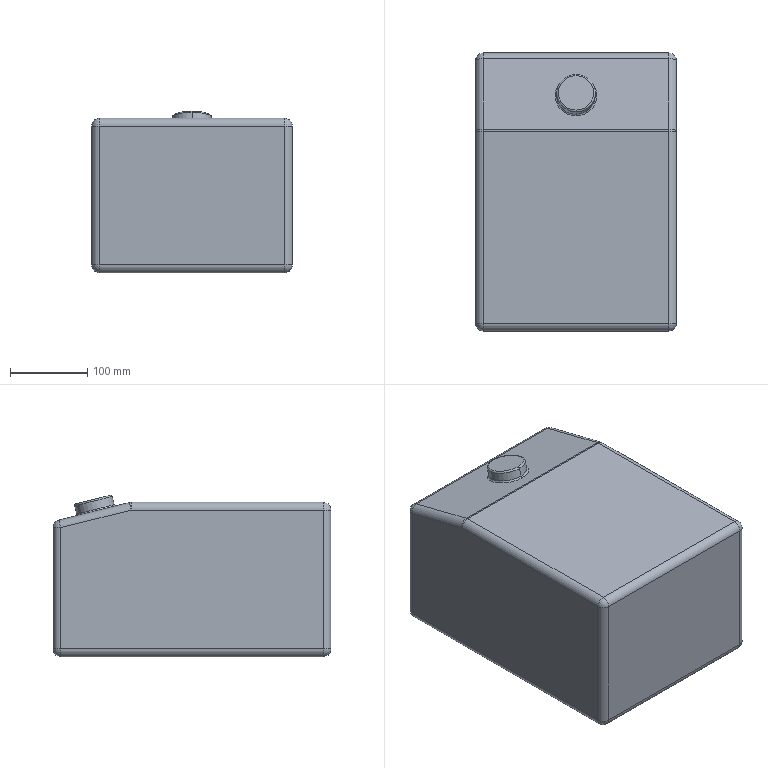Part | 1 solid | 39 faces | box 260 x 360 x 209.059 mm | volume 18358765 mm3 | cylinder 17 | sphere 10 | plane 8 | torus 4 | commonest cylinder face diameters 20 x15 50 x2
STEP:
#1=CARTESIAN_POINT('',(0.,151.932,195.417));
#2=VERTEX_POINT('',#1);
#3=CARTESIAN_POINT('',(0.,103.425,207.544));
#4=VERTEX_POINT('',#3);
#5=CARTESIAN_POINT('',(0.,127.678,201.481));
#6=DIRECTION('',(0.,-0.2425,-0.9701));
#7=DIRECTION('',(0.,-0.9701,0.2425));
#8=AXIS2_PLACEMENT_3D('',#5,#6,#7);
#9=CIRCLE('',#8,25.);
#10=EDGE_CURVE('',#2,#4,#9,.T.);
#11=ORIENTED_EDGE('',*,*,#10,.F.);
#12=CARTESIAN_POINT('',(0.,150.477,197.842));
#13=VERTEX_POINT('',#12);
#14=CARTESIAN_POINT('',(0.,149.992,195.902));
#15=DIRECTION('',(1.,0.,0.));
#16=DIRECTION('',(0.,1.,0.));
#17=AXIS2_PLACEMENT_3D('',#14,#15,#16);
#18=CIRCLE('',#17,2.);
#19=EDGE_CURVE('',#2,#13,#18,.T.);
#20=ORIENTED_EDGE('',*,*,#19,.T.);
#21=CARTESIAN_POINT('',(0.,105.85,208.999));
#22=VERTEX_POINT('',#21);
#23=CARTESIAN_POINT('',(0.,128.163,203.421));
#24=DIRECTION('',(0.,0.2425,0.9701));
#25=DIRECTION('',(0.,-0.9701,0.2425));
#26=AXIS2_PLACEMENT_3D('',#23,#24,#25);
#27=CIRCLE('',#26,23.);
#28=EDGE_CURVE('',#22,#13,#27,.T.);
#29=ORIENTED_EDGE('',*,*,#28,.F.);
#30=CARTESIAN_POINT('',(0.,105.365,207.059));
#31=DIRECTION('',(-1.,0.,0.));
#32=DIRECTION('',(0.,0.,1.));
#33=AXIS2_PLACEMENT_3D('',#30,#31,#32);
#34=CIRCLE('',#33,2.);
#35=EDGE_CURVE('',#4,#22,#34,.T.);
#36=ORIENTED_EDGE('',*,*,#35,.F.);
#37=EDGE_LOOP('',(#11,#20,#29,#36));
#38=FACE_OUTER_BOUND('',#37,.T.);
#39=CARTESIAN_POINT('',(0.,127.678,201.481));
#40=DIRECTION('',(0.,0.2425,0.9701));
#41=DIRECTION('',(0.,-0.9701,0.2425));
#42=AXIS2_PLACEMENT_3D('',#39,#40,#41);
#43=TOROIDAL_SURFACE('',#42,23.,2.);
#44=ADVANCED_FACE('',(#38),#43,.T.);
#45=CARTESIAN_POINT('',(0.,98.332,195.417));
#46=VERTEX_POINT('',#45);
#47=CARTESIAN_POINT('',(0.,150.719,182.32));
#48=VERTEX_POINT('',#47);
#49=CARTESIAN_POINT('',(0.,124.525,188.869));
#50=DIRECTION('',(0.,-0.2425,-0.9701));
#51=DIRECTION('',(0.,0.9701,-0.2425));
#52=AXIS2_PLACEMENT_3D('',#49,#50,#51);
#53=CIRCLE('',#52,27.);
#54=EDGE_CURVE('',#46,#48,#53,.T.);
#55=ORIENTED_EDGE('',*,*,#54,.F.);
#56=CARTESIAN_POINT('',(0.,100.757,196.872));
#57=VERTEX_POINT('',#56);
#58=CARTESIAN_POINT('',(0.,98.817,197.357));
#59=DIRECTION('',(1.,0.,0.));
#60=DIRECTION('',(0.,1.,0.));
#61=AXIS2_PLACEMENT_3D('',#58,#59,#60);
#62=CIRCLE('',#61,2.);
#63=EDGE_CURVE('',#46,#57,#62,.T.);
#64=ORIENTED_EDGE('',*,*,#63,.T.);
#65=CARTESIAN_POINT('',(0.,149.264,184.746));
#66=VERTEX_POINT('',#65);
#67=CARTESIAN_POINT('',(0.,125.01,190.809));
#68=DIRECTION('',(0.,0.2425,0.9701));
#69=DIRECTION('',(0.,0.9701,-0.2425));
#70=AXIS2_PLACEMENT_3D('',#67,#68,#69);
#71=CIRCLE('',#70,25.);
#72=EDGE_CURVE('',#66,#57,#71,.T.);
#73=ORIENTED_EDGE('',*,*,#72,.F.);
#74=CARTESIAN_POINT('',(0.,151.204,184.26));
#75=DIRECTION('',(-1.,0.,0.));
#76=DIRECTION('',(0.,0.,1.));
#77=AXIS2_PLACEMENT_3D('',#74,#75,#76);
#78=CIRCLE('',#77,2.);
#79=EDGE_CURVE('',#48,#66,#78,.T.);
#80=ORIENTED_EDGE('',*,*,#79,.F.);
#81=EDGE_LOOP('',(#55,#64,#73,#80));
#82=FACE_OUTER_BOUND('',#81,.T.);
#83=CARTESIAN_POINT('',(0.,125.01,190.809));
#84=DIRECTION('',(0.,-0.2425,-0.9701));
#85=DIRECTION('',(0.,0.9701,-0.2425));
#86=AXIS2_PLACEMENT_3D('',#83,#84,#85);
#87=TOROIDAL_SURFACE('',#86,27.,2.);
#88=ADVANCED_FACE('',(#82),#87,.F.);
#89=ORIENTED_EDGE('',*,*,#10,.T.);
#90=CARTESIAN_POINT('',(0.,103.91,209.484));
#91=DIRECTION('',(0.,-0.2425,-0.9701));
#92=VECTOR('',#91,1000.);
#93=LINE('',#90,#92);
#94=EDGE_CURVE('',#4,#57,#93,.T.);
#95=ORIENTED_EDGE('',*,*,#94,.T.);
#96=CARTESIAN_POINT('',(0.,125.01,190.809));
#97=DIRECTION('',(0.,0.2425,0.9701));
#98=DIRECTION('',(0.,0.9701,-0.2425));
#99=AXIS2_PLACEMENT_3D('',#96,#97,#98);
#100=CIRCLE('',#99,25.);
#101=EDGE_CURVE('',#57,#66,#100,.T.);
#102=ORIENTED_EDGE('',*,*,#101,.T.);
#103=CARTESIAN_POINT('',(0.,152.417,197.357));
#104=DIRECTION('',(0.,-0.2425,-0.9701));
#105=VECTOR('',#104,1000.);
#106=LINE('',#103,#105);
#107=EDGE_CURVE('',#2,#66,#106,.T.);
#108=ORIENTED_EDGE('',*,*,#107,.F.);
#109=EDGE_LOOP('',(#89,#95,#102,#108));
#110=FACE_OUTER_BOUND('',#109,.T.);
#111=CARTESIAN_POINT('',(0.,128.163,203.421));
#112=DIRECTION('',(0.,-0.2425,-0.9701));
#113=DIRECTION('',(0.,0.9701,-0.2425));
#114=AXIS2_PLACEMENT_3D('',#111,#112,#113);
#115=CYLINDRICAL_SURFACE('',#114,25.);
#116=ADVANCED_FACE('',(#110),#115,.T.);
#117=CARTESIAN_POINT('',(130.,-170.,10.));
#118=VERTEX_POINT('',#117);
#119=CARTESIAN_POINT('',(130.,170.,10.));
#120=VERTEX_POINT('',#119);
#121=CARTESIAN_POINT('',(130.,180.,10.));
#122=DIRECTION('',(0.,1.,0.));
#123=VECTOR('',#122,1000.);
#124=LINE('',#121,#123);
#125=EDGE_CURVE('',#118,#120,#124,.T.);
#126=ORIENTED_EDGE('',*,*,#125,.T.);
#127=CARTESIAN_POINT('',(130.,170.,167.192));
#128=VERTEX_POINT('',#127);
#129=CARTESIAN_POINT('',(130.,170.,200.));
#130=DIRECTION('',(0.,0.,1.));
#131=VECTOR('',#130,1000.);
#132=LINE('',#129,#131);
#133=EDGE_CURVE('',#120,#128,#132,.T.);
#134=ORIENTED_EDGE('',*,*,#133,.T.);
#135=CARTESIAN_POINT('',(130.,78.769,190.));
#136=VERTEX_POINT('',#135);
#137=CARTESIAN_POINT('',(130.,-167.131,251.475));
#138=DIRECTION('',(0.,-0.9701,0.2425));
#139=VECTOR('',#138,1000.);
#140=LINE('',#137,#139);
#141=EDGE_CURVE('',#128,#136,#140,.T.);
#142=ORIENTED_EDGE('',*,*,#141,.T.);
#143=CARTESIAN_POINT('',(130.,-170.,190.));
#144=VERTEX_POINT('',#143);
#145=CARTESIAN_POINT('',(130.,-180.,190.));
#146=DIRECTION('',(0.,-1.,0.));
#147=VECTOR('',#146,1000.);
#148=LINE('',#145,#147);
#149=EDGE_CURVE('',#136,#144,#148,.T.);
#150=ORIENTED_EDGE('',*,*,#149,.T.);
#151=CARTESIAN_POINT('',(130.,-170.,200.));
#152=DIRECTION('',(0.,0.,-1.));
#153=VECTOR('',#152,1000.);
#154=LINE('',#151,#153);
#155=EDGE_CURVE('',#144,#118,#154,.T.);
#156=ORIENTED_EDGE('',*,*,#155,.T.);
#157=EDGE_LOOP('',(#126,#134,#142,#150,#156));
#158=FACE_OUTER_BOUND('',#157,.T.);
#159=CARTESIAN_POINT('',(130.,-180.,200.));
#160=DIRECTION('',(-1.,0.,0.));
#161=DIRECTION('',(0.,0.,1.));
#162=AXIS2_PLACEMENT_3D('',#159,#160,#161);
#163=PLANE('',#162);
#164=ADVANCED_FACE('',(#158),#163,.F.);
#165=CARTESIAN_POINT('',(-120.,180.,167.192));
#166=VERTEX_POINT('',#165);
#167=CARTESIAN_POINT('',(120.,180.,167.192));
#168=VERTEX_POINT('',#167);
#169=CARTESIAN_POINT('',(-130.,180.,167.192));
#170=DIRECTION('',(1.,0.,0.));
#171=VECTOR('',#170,1000.);
#172=LINE('',#169,#171);
#173=EDGE_CURVE('',#166,#168,#172,.T.);
#174=ORIENTED_EDGE('',*,*,#173,.T.);
#175=CARTESIAN_POINT('',(120.,180.,10.));
#176=VERTEX_POINT('',#175);
#177=CARTESIAN_POINT('',(120.,180.,200.));
#178=DIRECTION('',(0.,0.,-1.));
#179=VECTOR('',#178,1000.);
#180=LINE('',#177,#179);
#181=EDGE_CURVE('',#168,#176,#180,.T.);
#182=ORIENTED_EDGE('',*,*,#181,.T.);
#183=CARTESIAN_POINT('',(-120.,180.,10.));
#184=VERTEX_POINT('',#183);
#185=CARTESIAN_POINT('',(-130.,180.,10.));
#186=DIRECTION('',(-1.,0.,0.));
#187=VECTOR('',#186,1000.);
#188=LINE('',#185,#187);
#189=EDGE_CURVE('',#176,#184,#188,.T.);
#190=ORIENTED_EDGE('',*,*,#189,.T.);
#191=CARTESIAN_POINT('',(-120.,180.,200.));
#192=DIRECTION('',(0.,0.,1.));
#193=VECTOR('',#192,1000.);
#194=LINE('',#191,#193);
#195=EDGE_CURVE('',#184,#166,#194,.T.);
#196=ORIENTED_EDGE('',*,*,#195,.T.);
#197=EDGE_LOOP('',(#174,#182,#190,#196));
#198=FACE_OUTER_BOUND('',#197,.T.);
#199=CARTESIAN_POINT('',(-130.,180.,200.));
#200=DIRECTION('',(0.,-1.,0.));
#201=DIRECTION('',(0.,0.,-1.));
#202=AXIS2_PLACEMENT_3D('',#199,#200,#201);
#203=PLANE('',#202);
#204=ADVANCED_FACE('',(#198),#203,.F.);
#205=CARTESIAN_POINT('',(-130.,170.,10.));
#206=VERTEX_POINT('',#205);
#207=CARTESIAN_POINT('',(-130.,-170.,10.));
#208=VERTEX_POINT('',#207);
#209=CARTESIAN_POINT('',(-130.,-180.,10.));
#210=DIRECTION('',(0.,-1.,0.));
#211=VECTOR('',#210,1000.);
#212=LINE('',#209,#211);
#213=EDGE_CURVE('',#206,#208,#212,.T.);
#214=ORIENTED_EDGE('',*,*,#213,.T.);
#215=CARTESIAN_POINT('',(-130.,-170.,190.));
#216=VERTEX_POINT('',#215);
#217=CARTESIAN_POINT('',(-130.,-170.,200.));
#218=DIRECTION('',(0.,0.,1.));
#219=VECTOR('',#218,1000.);
#220=LINE('',#217,#219);
#221=EDGE_CURVE('',#208,#216,#220,.T.);
#222=ORIENTED_EDGE('',*,*,#221,.T.);
#223=CARTESIAN_POINT('',(-130.,78.769,190.));
#224=VERTEX_POINT('',#223);
#225=CARTESIAN_POINT('',(-130.,-180.,190.));
#226=DIRECTION('',(0.,1.,0.));
#227=VECTOR('',#226,1000.);
#228=LINE('',#225,#227);
#229=EDGE_CURVE('',#216,#224,#228,.T.);
#230=ORIENTED_EDGE('',*,*,#229,.T.);
#231=CARTESIAN_POINT('',(-130.,170.,167.192));
#232=VERTEX_POINT('',#231);
#233=CARTESIAN_POINT('',(-130.,-167.131,251.475));
#234=DIRECTION('',(0.,0.9701,-0.2425));
#235=VECTOR('',#234,1000.);
#236=LINE('',#233,#235);
#237=EDGE_CURVE('',#224,#232,#236,.T.);
#238=ORIENTED_EDGE('',*,*,#237,.T.);
#239=CARTESIAN_POINT('',(-130.,170.,200.));
#240=DIRECTION('',(0.,0.,-1.));
#241=VECTOR('',#240,1000.);
#242=LINE('',#239,#241);
#243=EDGE_CURVE('',#232,#206,#242,.T.);
#244=ORIENTED_EDGE('',*,*,#243,.T.);
#245=EDGE_LOOP('',(#214,#222,#230,#238,#244));
#246=FACE_OUTER_BOUND('',#245,.T.);
#247=CARTESIAN_POINT('',(-130.,-180.,200.));
#248=DIRECTION('',(1.,0.,0.));
#249=DIRECTION('',(0.,0.,-1.));
#250=AXIS2_PLACEMENT_3D('',#247,#248,#249);
#251=PLANE('',#250);
#252=ADVANCED_FACE('',(#246),#251,.F.);
#253=CARTESIAN_POINT('',(120.,-180.,190.));
#254=VERTEX_POINT('',#253);
#255=CARTESIAN_POINT('',(-120.,-180.,190.));
#256=VERTEX_POINT('',#255);
#257=CARTESIAN_POINT('',(-130.,-180.,190.));
#258=DIRECTION('',(-1.,0.,0.));
#259=VECTOR('',#258,1000.);
#260=LINE('',#257,#259);
#261=EDGE_CURVE('',#254,#256,#260,.T.);
#262=ORIENTED_EDGE('',*,*,#261,.T.);
#263=CARTESIAN_POINT('',(-120.,-180.,10.));
#264=VERTEX_POINT('',#263);
#265=CARTESIAN_POINT('',(-120.,-180.,200.));
#266=DIRECTION('',(0.,0.,-1.));
#267=VECTOR('',#266,1000.);
#268=LINE('',#265,#267);
#269=EDGE_CURVE('',#256,#264,#268,.T.);
#270=ORIENTED_EDGE('',*,*,#269,.T.);
#271=CARTESIAN_POINT('',(120.,-180.,10.));
#272=VERTEX_POINT('',#271);
#273=CARTESIAN_POINT('',(130.,-180.,10.));
#274=DIRECTION('',(1.,0.,0.));
#275=VECTOR('',#274,1000.);
#276=LINE('',#273,#275);
#277=EDGE_CURVE('',#264,#272,#276,.T.);
#278=ORIENTED_EDGE('',*,*,#277,.T.);
#279=CARTESIAN_POINT('',(120.,-180.,200.));
#280=DIRECTION('',(0.,0.,1.));
#281=VECTOR('',#280,1000.);
#282=LINE('',#279,#281);
#283=EDGE_CURVE('',#272,#254,#282,.T.);
#284=ORIENTED_EDGE('',*,*,#283,.T.);
#285=EDGE_LOOP('',(#262,#270,#278,#284));
#286=FACE_OUTER_BOUND('',#285,.T.);
#287=CARTESIAN_POINT('',(-130.,-180.,200.));
#288=DIRECTION('',(0.,1.,0.));
#289=DIRECTION('',(0.,0.,1.));
#290=AXIS2_PLACEMENT_3D('',#287,#288,#289);
#291=PLANE('',#290);
#292=ADVANCED_FACE('',(#286),#291,.F.);
#293=CARTESIAN_POINT('',(-120.,78.769,200.));
#294=VERTEX_POINT('',#293);
#295=CARTESIAN_POINT('',(-120.,-170.,200.));
#296=VERTEX_POINT('',#295);
#297=CARTESIAN_POINT('',(-120.,0.,200.));
#298=DIRECTION('',(0.,-1.,0.));
#299=VECTOR('',#298,1000.);
#300=LINE('',#297,#299);
#301=EDGE_CURVE('',#294,#296,#300,.T.);
#302=ORIENTED_EDGE('',*,*,#301,.T.);
#303=CARTESIAN_POINT('',(120.,-170.,200.));
#304=VERTEX_POINT('',#303);
#305=CARTESIAN_POINT('',(0.,-170.,200.));
#306=DIRECTION('',(1.,0.,0.));
#307=VECTOR('',#306,1000.);
#308=LINE('',#305,#307);
#309=EDGE_CURVE('',#296,#304,#308,.T.);
#310=ORIENTED_EDGE('',*,*,#309,.T.);
#311=CARTESIAN_POINT('',(120.,78.769,200.));
#312=VERTEX_POINT('',#311);
#313=CARTESIAN_POINT('',(120.,0.,200.));
#314=DIRECTION('',(0.,1.,0.));
#315=VECTOR('',#314,1000.);
#316=LINE('',#313,#315);
#317=EDGE_CURVE('',#304,#312,#316,.T.);
#318=ORIENTED_EDGE('',*,*,#317,.T.);
#319=CARTESIAN_POINT('',(0.,78.769,200.));
#320=DIRECTION('',(-1.,0.,0.));
#321=VECTOR('',#320,1000.);
#322=LINE('',#319,#321);
#323=EDGE_CURVE('',#312,#294,#322,.T.);
#324=ORIENTED_EDGE('',*,*,#323,.T.);
#325=EDGE_LOOP('',(#302,#310,#318,#324));
#326=FACE_OUTER_BOUND('',#325,.T.);
#327=CARTESIAN_POINT('',(0.,0.,200.));
#328=DIRECTION('',(0.,0.,-1.));
#329=DIRECTION('',(-1.,0.,0.));
#330=AXIS2_PLACEMENT_3D('',#327,#328,#329);
#331=PLANE('',#330);
#332=ADVANCED_FACE('',(#326),#331,.F.);
#333=CARTESIAN_POINT('',(-120.,-170.,0.));
#334=VERTEX_POINT('',#333);
#335=CARTESIAN_POINT('',(-120.,170.,0.));
#336=VERTEX_POINT('',#335);
#337=CARTESIAN_POINT('',(-120.,180.,0.));
#338=DIRECTION('',(0.,1.,0.));
#339=VECTOR('',#338,1000.);
#340=LINE('',#337,#339);
#341=EDGE_CURVE('',#334,#336,#340,.T.);
#342=ORIENTED_EDGE('',*,*,#341,.T.);
#343=CARTESIAN_POINT('',(120.,170.,0.));
#344=VERTEX_POINT('',#343);
#345=CARTESIAN_POINT('',(130.,170.,0.));
#346=DIRECTION('',(1.,0.,0.));
#347=VECTOR('',#346,1000.);
#348=LINE('',#345,#347);
#349=EDGE_CURVE('',#336,#344,#348,.T.);
#350=ORIENTED_EDGE('',*,*,#349,.T.);
#351=CARTESIAN_POINT('',(120.,-170.,0.));
#352=VERTEX_POINT('',#351);
#353=CARTESIAN_POINT('',(120.,-180.,0.));
#354=DIRECTION('',(0.,-1.,0.));
#355=VECTOR('',#354,1000.);
#356=LINE('',#353,#355);
#357=EDGE_CURVE('',#344,#352,#356,.T.);
#358=ORIENTED_EDGE('',*,*,#357,.T.);
#359=CARTESIAN_POINT('',(-130.,-170.,0.));
#360=DIRECTION('',(-1.,0.,0.));
#361=VECTOR('',#360,1000.);
#362=LINE('',#359,#361);
#363=EDGE_CURVE('',#352,#334,#362,.T.);
#364=ORIENTED_EDGE('',*,*,#363,.T.);
#365=EDGE_LOOP('',(#342,#350,#358,#364));
#366=FACE_OUTER_BOUND('',#365,.T.);
#367=CARTESIAN_POINT('',(0.,0.,0.));
#368=DIRECTION('',(0.,0.,-1.));
#369=DIRECTION('',(-1.,0.,0.));
#370=AXIS2_PLACEMENT_3D('',#367,#368,#369);
#371=PLANE('',#370);
#372=ADVANCED_FACE('',(#366),#371,.T.);
#373=CARTESIAN_POINT('',(-120.,81.194,199.701));
#374=VERTEX_POINT('',#373);
#375=CARTESIAN_POINT('',(120.,81.194,199.701));
#376=VERTEX_POINT('',#375);
#377=CARTESIAN_POINT('',(130.,81.194,199.701));
#378=DIRECTION('',(1.,0.,0.));
#379=VECTOR('',#378,1000.);
#380=LINE('',#377,#379);
#381=EDGE_CURVE('',#374,#376,#380,.T.);
#382=ORIENTED_EDGE('',*,*,#381,.T.);
#383=CARTESIAN_POINT('',(120.,172.425,176.894));
#384=VERTEX_POINT('',#383);
#385=CARTESIAN_POINT('',(120.,180.,175.));
#386=DIRECTION('',(0.,0.9701,-0.2425));
#387=VECTOR('',#386,1000.);
#388=LINE('',#385,#387);
#389=EDGE_CURVE('',#376,#384,#388,.T.);
#390=ORIENTED_EDGE('',*,*,#389,.T.);
#391=CARTESIAN_POINT('',(-120.,172.425,176.894));
#392=VERTEX_POINT('',#391);
#393=CARTESIAN_POINT('',(130.,172.425,176.894));
#394=DIRECTION('',(-1.,0.,0.));
#395=VECTOR('',#394,1000.);
#396=LINE('',#393,#395);
#397=EDGE_CURVE('',#384,#392,#396,.T.);
#398=ORIENTED_EDGE('',*,*,#397,.T.);
#399=CARTESIAN_POINT('',(-120.,180.,175.));
#400=DIRECTION('',(0.,-0.9701,0.2425));
#401=VECTOR('',#400,1000.);
#402=LINE('',#399,#401);
#403=EDGE_CURVE('',#392,#374,#402,.T.);
#404=ORIENTED_EDGE('',*,*,#403,.T.);
#405=EDGE_LOOP('',(#382,#390,#398,#404));
#406=FACE_OUTER_BOUND('',#405,.T.);
#407=CARTESIAN_POINT('',(0.,124.525,188.869));
#408=DIRECTION('',(0.,-0.2425,-0.9701));
#409=DIRECTION('',(0.,0.9701,-0.2425));
#410=AXIS2_PLACEMENT_3D('',#407,#408,#409);
#411=CIRCLE('',#410,27.);
#412=EDGE_CURVE('',#48,#46,#411,.T.);
#413=ORIENTED_EDGE('',*,*,#412,.T.);
#414=ORIENTED_EDGE('',*,*,#54,.T.);
#415=EDGE_LOOP('',(#413,#414));
#416=FACE_BOUND('',#415,.T.);
#417=CARTESIAN_POINT('',(130.,180.,175.));
#418=DIRECTION('',(0.,-0.2425,-0.9701));
#419=DIRECTION('',(0.,0.9701,-0.2425));
#420=AXIS2_PLACEMENT_3D('',#417,#418,#419);
#421=PLANE('',#420);
#422=ADVANCED_FACE('',(#406,#416),#421,.F.);
#423=ORIENTED_EDGE('',*,*,#277,.F.);
#424=CARTESIAN_POINT('',(-120.,-170.,10.));
#425=DIRECTION('',(1.,0.,0.));
#426=DIRECTION('',(0.,0.,1.));
#427=AXIS2_PLACEMENT_3D('',#424,#425,#426);
#428=CIRCLE('',#427,10.);
#429=EDGE_CURVE('',#264,#334,#428,.T.);
#430=ORIENTED_EDGE('',*,*,#429,.T.);
#431=ORIENTED_EDGE('',*,*,#363,.F.);
#432=CARTESIAN_POINT('',(120.,-170.,10.));
#433=DIRECTION('',(-1.,0.,0.));
#434=DIRECTION('',(0.,0.,1.));
#435=AXIS2_PLACEMENT_3D('',#432,#433,#434);
#436=CIRCLE('',#435,10.);
#437=EDGE_CURVE('',#352,#272,#436,.T.);
#438=ORIENTED_EDGE('',*,*,#437,.T.);
#439=EDGE_LOOP('',(#423,#430,#431,#438));
#440=FACE_OUTER_BOUND('',#439,.T.);
#441=CARTESIAN_POINT('',(-130.,-170.,10.));
#442=DIRECTION('',(-1.,0.,0.));
#443=DIRECTION('',(0.,0.,1.));
#444=AXIS2_PLACEMENT_3D('',#441,#442,#443);
#445=CYLINDRICAL_SURFACE('',#444,10.);
#446=ADVANCED_FACE('',(#440),#445,.T.);
#447=ORIENTED_EDGE('',*,*,#125,.F.);
#448=CARTESIAN_POINT('',(120.,-170.,10.));
#449=DIRECTION('',(0.,1.,0.));
#450=DIRECTION('',(0.,0.,-1.));
#451=AXIS2_PLACEMENT_3D('',#448,#449,#450);
#452=CIRCLE('',#451,10.);
#453=EDGE_CURVE('',#118,#352,#452,.T.);
#454=ORIENTED_EDGE('',*,*,#453,.T.);
#455=ORIENTED_EDGE('',*,*,#357,.F.);
#456=CARTESIAN_POINT('',(120.,170.,10.));
#457=DIRECTION('',(0.,-1.,0.));
#458=DIRECTION('',(0.,0.,-1.));
#459=AXIS2_PLACEMENT_3D('',#456,#457,#458);
#460=CIRCLE('',#459,10.);
#461=EDGE_CURVE('',#344,#120,#460,.T.);
#462=ORIENTED_EDGE('',*,*,#461,.T.);
#463=EDGE_LOOP('',(#447,#454,#455,#462));
#464=FACE_OUTER_BOUND('',#463,.T.);
#465=CARTESIAN_POINT('',(120.,-180.,10.));
#466=DIRECTION('',(0.,-1.,0.));
#467=DIRECTION('',(0.,0.,-1.));
#468=AXIS2_PLACEMENT_3D('',#465,#466,#467);
#469=CYLINDRICAL_SURFACE('',#468,10.);
#470=ADVANCED_FACE('',(#464),#469,.T.);
#471=ORIENTED_EDGE('',*,*,#341,.F.);
#472=CARTESIAN_POINT('',(-120.,-170.,10.));
#473=DIRECTION('',(0.,1.,0.));
#474=DIRECTION('',(0.,0.,1.));
#475=AXIS2_PLACEMENT_3D('',#472,#473,#474);
#476=CIRCLE('',#475,10.);
#477=EDGE_CURVE('',#334,#208,#476,.T.);
#478=ORIENTED_EDGE('',*,*,#477,.T.);
#479=ORIENTED_EDGE('',*,*,#213,.F.);
#480=CARTESIAN_POINT('',(-120.,170.,10.));
#481=DIRECTION('',(0.,-1.,0.));
#482=DIRECTION('',(0.,0.,1.));
#483=AXIS2_PLACEMENT_3D('',#480,#481,#482);
#484=CIRCLE('',#483,10.);
#485=EDGE_CURVE('',#206,#336,#484,.T.);
#486=ORIENTED_EDGE('',*,*,#485,.T.);
#487=EDGE_LOOP('',(#471,#478,#479,#486));
#488=FACE_OUTER_BOUND('',#487,.T.);
#489=CARTESIAN_POINT('',(-120.,-180.,10.));
#490=DIRECTION('',(0.,1.,0.));
#491=DIRECTION('',(0.,0.,1.));
#492=AXIS2_PLACEMENT_3D('',#489,#490,#491);
#493=CYLINDRICAL_SURFACE('',#492,10.);
#494=ADVANCED_FACE('',(#488),#493,.T.);
#495=ORIENTED_EDGE('',*,*,#189,.F.);
#496=CARTESIAN_POINT('',(120.,170.,10.));
#497=DIRECTION('',(-1.,0.,0.));
#498=DIRECTION('',(0.,0.,-1.));
#499=AXIS2_PLACEMENT_3D('',#496,#497,#498);
#500=CIRCLE('',#499,10.);
#501=EDGE_CURVE('',#176,#344,#500,.T.);
#502=ORIENTED_EDGE('',*,*,#501,.T.);
#503=ORIENTED_EDGE('',*,*,#349,.F.);
#504=CARTESIAN_POINT('',(-120.,170.,10.));
#505=DIRECTION('',(1.,0.,0.));
#506=DIRECTION('',(0.,0.,-1.));
#507=AXIS2_PLACEMENT_3D('',#504,#505,#506);
#508=CIRCLE('',#507,10.);
#509=EDGE_CURVE('',#336,#184,#508,.T.);
#510=ORIENTED_EDGE('',*,*,#509,.T.);
#511=EDGE_LOOP('',(#495,#502,#503,#510));
#512=FACE_OUTER_BOUND('',#511,.T.);
#513=CARTESIAN_POINT('',(-130.,170.,10.));
#514=DIRECTION('',(1.,0.,0.));
#515=DIRECTION('',(0.,0.,-1.));
#516=AXIS2_PLACEMENT_3D('',#513,#514,#515);
#517=CYLINDRICAL_SURFACE('',#516,10.);
#518=ADVANCED_FACE('',(#512),#517,.T.);
#519=ORIENTED_EDGE('',*,*,#94,.F.);
#520=CARTESIAN_POINT('',(0.,127.678,201.481));
#521=DIRECTION('',(0.,-0.2425,-0.9701));
#522=DIRECTION('',(0.,-0.9701,0.2425));
#523=AXIS2_PLACEMENT_3D('',#520,#521,#522);
#524=CIRCLE('',#523,25.);
#525=EDGE_CURVE('',#4,#2,#524,.T.);
#526=ORIENTED_EDGE('',*,*,#525,.T.);
#527=ORIENTED_EDGE('',*,*,#107,.T.);
#528=ORIENTED_EDGE('',*,*,#72,.T.);
#529=EDGE_LOOP('',(#519,#526,#527,#528));
#530=FACE_OUTER_BOUND('',#529,.T.);
#531=CARTESIAN_POINT('',(0.,128.163,203.421));
#532=DIRECTION('',(0.,-0.2425,-0.9701));
#533=DIRECTION('',(0.,0.9701,-0.2425));
#534=AXIS2_PLACEMENT_3D('',#531,#532,#533);
#535=CYLINDRICAL_SURFACE('',#534,25.);
#536=ADVANCED_FACE('',(#530),#535,.T.);
#537=ORIENTED_EDGE('',*,*,#28,.T.);
#538=CARTESIAN_POINT('',(0.,128.163,203.421));
#539=DIRECTION('',(0.,0.2425,0.9701));
#540=DIRECTION('',(0.,-0.9701,0.2425));
#541=AXIS2_PLACEMENT_3D('',#538,#539,#540);
#542=CIRCLE('',#541,23.);
#543=EDGE_CURVE('',#13,#22,#542,.T.);
#544=ORIENTED_EDGE('',*,*,#543,.T.);
#545=EDGE_LOOP('',(#537,#544));
#546=FACE_OUTER_BOUND('',#545,.T.);
#547=CARTESIAN_POINT('',(0.,128.163,203.421));
#548=DIRECTION('',(0.,0.2425,0.9701));
#549=DIRECTION('',(0.,-0.9701,0.2425));
#550=AXIS2_PLACEMENT_3D('',#547,#548,#549);
#551=PLANE('',#550);
#552=ADVANCED_FACE('',(#546),#551,.T.);
#553=ORIENTED_EDGE('',*,*,#63,.F.);
#554=ORIENTED_EDGE('',*,*,#412,.F.);
#555=ORIENTED_EDGE('',*,*,#79,.T.);
#556=ORIENTED_EDGE('',*,*,#101,.F.);
#557=EDGE_LOOP('',(#553,#554,#555,#556));
#558=FACE_OUTER_BOUND('',#557,.T.);
#559=CARTESIAN_POINT('',(0.,125.01,190.809));
#560=DIRECTION('',(0.,-0.2425,-0.9701));
#561=DIRECTION('',(0.,0.9701,-0.2425));
#562=AXIS2_PLACEMENT_3D('',#559,#560,#561);
#563=TOROIDAL_SURFACE('',#562,27.,2.);
#564=ADVANCED_FACE('',(#558),#563,.F.);
#565=ORIENTED_EDGE('',*,*,#19,.F.);
#566=ORIENTED_EDGE('',*,*,#525,.F.);
#567=ORIENTED_EDGE('',*,*,#35,.T.);
#568=ORIENTED_EDGE('',*,*,#543,.F.);
#569=EDGE_LOOP('',(#565,#566,#567,#568));
#570=FACE_OUTER_BOUND('',#569,.T.);
#571=CARTESIAN_POINT('',(0.,127.678,201.481));
#572=DIRECTION('',(0.,0.2425,0.9701));
#573=DIRECTION('',(0.,-0.9701,0.2425));
#574=AXIS2_PLACEMENT_3D('',#571,#572,#573);
#575=TOROIDAL_SURFACE('',#574,23.,2.);
#576=ADVANCED_FACE('',(#570),#575,.T.);
#577=ORIENTED_EDGE('',*,*,#461,.F.);
#578=ORIENTED_EDGE('',*,*,#501,.F.);
#579=CARTESIAN_POINT('',(120.,170.,10.));
#580=DIRECTION('',(0.,0.,1.));
#581=DIRECTION('',(1.,0.,0.));
#582=AXIS2_PLACEMENT_3D('',#579,#580,#581);
#583=CIRCLE('',#582,10.);
#584=EDGE_CURVE('',#120,#176,#583,.T.);
#585=ORIENTED_EDGE('',*,*,#584,.F.);
#586=EDGE_LOOP('',(#577,#578,#585));
#587=FACE_OUTER_BOUND('',#586,.T.);
#588=CARTESIAN_POINT('',(120.,170.,10.));
#589=DIRECTION('',(0.,1.,0.));
#590=DIRECTION('',(1.,0.,0.));
#591=AXIS2_PLACEMENT_3D('',#588,#589,#590);
#592=SPHERICAL_SURFACE('',#591,10.);
#593=ADVANCED_FACE('',(#587),#592,.T.);
#594=ORIENTED_EDGE('',*,*,#584,.T.);
#595=ORIENTED_EDGE('',*,*,#181,.F.);
#596=CARTESIAN_POINT('',(120.,170.,167.192));
#597=DIRECTION('',(0.,0.,1.));
#598=DIRECTION('',(1.,0.,0.));
#599=AXIS2_PLACEMENT_3D('',#596,#597,#598);
#600=CIRCLE('',#599,10.);
#601=EDGE_CURVE('',#128,#168,#600,.T.);
#602=ORIENTED_EDGE('',*,*,#601,.F.);
#603=ORIENTED_EDGE('',*,*,#133,.F.);
#604=EDGE_LOOP('',(#594,#595,#602,#603));
#605=FACE_OUTER_BOUND('',#604,.T.);
#606=CARTESIAN_POINT('',(120.,170.,200.));
#607=DIRECTION('',(0.,0.,-1.));
#608=DIRECTION('',(-1.,0.,0.));
#609=AXIS2_PLACEMENT_3D('',#606,#607,#608);
#610=CYLINDRICAL_SURFACE('',#609,10.);
#611=ADVANCED_FACE('',(#605),#610,.T.);
#612=ORIENTED_EDGE('',*,*,#509,.F.);
#613=ORIENTED_EDGE('',*,*,#485,.F.);
#614=CARTESIAN_POINT('',(-120.,170.,10.));
#615=DIRECTION('',(0.,0.,1.));
#616=DIRECTION('',(1.,0.,0.));
#617=AXIS2_PLACEMENT_3D('',#614,#615,#616);
#618=CIRCLE('',#617,10.);
#619=EDGE_CURVE('',#184,#206,#618,.T.);
#620=ORIENTED_EDGE('',*,*,#619,.F.);
#621=EDGE_LOOP('',(#612,#613,#620));
#622=FACE_OUTER_BOUND('',#621,.T.);
#623=CARTESIAN_POINT('',(-120.,170.,10.));
#624=DIRECTION('',(0.,1.,0.));
#625=DIRECTION('',(1.,0.,0.));
#626=AXIS2_PLACEMENT_3D('',#623,#624,#625);
#627=SPHERICAL_SURFACE('',#626,10.);
#628=ADVANCED_FACE('',(#622),#627,.T.);
#629=CARTESIAN_POINT('',(120.,170.,167.192));
#630=DIRECTION('',(0.,-0.9701,0.2425));
#631=DIRECTION('',(0.,0.2425,0.9701));
#632=AXIS2_PLACEMENT_3D('',#629,#630,#631);
#633=CIRCLE('',#632,10.);
#634=EDGE_CURVE('',#128,#384,#633,.T.);
#635=ORIENTED_EDGE('',*,*,#634,.F.);
#636=ORIENTED_EDGE('',*,*,#601,.T.);
#637=CARTESIAN_POINT('',(120.,170.,167.192));
#638=DIRECTION('',(-1.,0.,0.));
#639=DIRECTION('',(0.,0.,-1.));
#640=AXIS2_PLACEMENT_3D('',#637,#638,#639);
#641=CIRCLE('',#640,10.);
#642=EDGE_CURVE('',#384,#168,#641,.T.);
#643=ORIENTED_EDGE('',*,*,#642,.F.);
#644=EDGE_LOOP('',(#635,#636,#643));
#645=FACE_OUTER_BOUND('',#644,.T.);
#646=CARTESIAN_POINT('',(120.,170.,167.192));
#647=DIRECTION('',(0.,1.,0.));
#648=DIRECTION('',(1.,0.,0.));
#649=AXIS2_PLACEMENT_3D('',#646,#647,#648);
#650=SPHERICAL_SURFACE('',#649,10.);
#651=ADVANCED_FACE('',(#645),#650,.T.);
#652=ORIENTED_EDGE('',*,*,#619,.T.);
#653=ORIENTED_EDGE('',*,*,#243,.F.);
#654=CARTESIAN_POINT('',(-120.,170.,167.192));
#655=DIRECTION('',(0.,0.,1.));
#656=DIRECTION('',(1.,0.,0.));
#657=AXIS2_PLACEMENT_3D('',#654,#655,#656);
#658=CIRCLE('',#657,10.);
#659=EDGE_CURVE('',#166,#232,#658,.T.);
#660=ORIENTED_EDGE('',*,*,#659,.F.);
#661=ORIENTED_EDGE('',*,*,#195,.F.);
#662=EDGE_LOOP('',(#652,#653,#660,#661));
#663=FACE_OUTER_BOUND('',#662,.T.);
#664=CARTESIAN_POINT('',(-120.,170.,200.));
#665=DIRECTION('',(0.,0.,-1.));
#666=DIRECTION('',(-1.,0.,0.));
#667=AXIS2_PLACEMENT_3D('',#664,#665,#666);
#668=CYLINDRICAL_SURFACE('',#667,10.);
#669=ADVANCED_FACE('',(#663),#668,.T.);
#670=ORIENTED_EDGE('',*,*,#642,.T.);
#671=ORIENTED_EDGE('',*,*,#173,.F.);
#672=CARTESIAN_POINT('',(-120.,170.,167.192));
#673=DIRECTION('',(-1.,0.,0.));
#674=DIRECTION('',(0.,-1.,0.));
#675=AXIS2_PLACEMENT_3D('',#672,#673,#674);
#676=CIRCLE('',#675,10.);
#677=EDGE_CURVE('',#392,#166,#676,.T.);
#678=ORIENTED_EDGE('',*,*,#677,.F.);
#679=ORIENTED_EDGE('',*,*,#397,.F.);
#680=EDGE_LOOP('',(#670,#671,#678,#679));
#681=FACE_OUTER_BOUND('',#680,.T.);
#682=CARTESIAN_POINT('',(130.,170.,167.192));
#683=DIRECTION('',(-1.,0.,0.));
#684=DIRECTION('',(0.,0.,1.));
#685=AXIS2_PLACEMENT_3D('',#682,#683,#684);
#686=CYLINDRICAL_SURFACE('',#685,10.);
#687=ADVANCED_FACE('',(#681),#686,.T.);
#688=ORIENTED_EDGE('',*,*,#634,.T.);
#689=ORIENTED_EDGE('',*,*,#389,.F.);
#690=CARTESIAN_POINT('',(120.,78.769,190.));
#691=DIRECTION('',(0.,-0.9701,0.2425));
#692=DIRECTION('',(0.,-0.2425,-0.9701));
#693=AXIS2_PLACEMENT_3D('',#690,#691,#692);
#694=CIRCLE('',#693,10.);
#695=EDGE_CURVE('',#136,#376,#694,.T.);
#696=ORIENTED_EDGE('',*,*,#695,.F.);
#697=ORIENTED_EDGE('',*,*,#141,.F.);
#698=EDGE_LOOP('',(#688,#689,#696,#697));
#699=FACE_OUTER_BOUND('',#698,.T.);
#700=CARTESIAN_POINT('',(120.,-167.131,251.475));
#701=DIRECTION('',(0.,-0.9701,0.2425));
#702=DIRECTION('',(0.,-0.2425,-0.9701));
#703=AXIS2_PLACEMENT_3D('',#700,#701,#702);
#704=CYLINDRICAL_SURFACE('',#703,10.);
#705=ADVANCED_FACE('',(#699),#704,.T.);
#706=ORIENTED_EDGE('',*,*,#677,.T.);
#707=ORIENTED_EDGE('',*,*,#659,.T.);
#708=CARTESIAN_POINT('',(-120.,170.,167.192));
#709=DIRECTION('',(0.,-0.9701,0.2425));
#710=DIRECTION('',(0.,0.2425,0.9701));
#711=AXIS2_PLACEMENT_3D('',#708,#709,#710);
#712=CIRCLE('',#711,10.);
#713=EDGE_CURVE('',#392,#232,#712,.T.);
#714=ORIENTED_EDGE('',*,*,#713,.F.);
#715=EDGE_LOOP('',(#706,#707,#714));
#716=FACE_OUTER_BOUND('',#715,.T.);
#717=CARTESIAN_POINT('',(-120.,170.,167.192));
#718=DIRECTION('',(0.,1.,0.));
#719=DIRECTION('',(1.,0.,0.));
#720=AXIS2_PLACEMENT_3D('',#717,#718,#719);
#721=SPHERICAL_SURFACE('',#720,10.);
#722=ADVANCED_FACE('',(#716),#721,.T.);
#723=CARTESIAN_POINT('',(120.,78.769,190.));
#724=DIRECTION('',(0.,-1.,0.));
#725=DIRECTION('',(-1.,0.,0.));
#726=AXIS2_PLACEMENT_3D('',#723,#724,#725);
#727=CIRCLE('',#726,10.);
#728=EDGE_CURVE('',#136,#312,#727,.T.);
#729=ORIENTED_EDGE('',*,*,#728,.F.);
#730=ORIENTED_EDGE('',*,*,#695,.T.);
#731=CARTESIAN_POINT('',(120.,78.769,190.));
#732=DIRECTION('',(-1.,0.,0.));
#733=DIRECTION('',(0.,0.,-1.));
#734=AXIS2_PLACEMENT_3D('',#731,#732,#733);
#735=CIRCLE('',#734,10.);
#736=EDGE_CURVE('',#312,#376,#735,.T.);
#737=ORIENTED_EDGE('',*,*,#736,.F.);
#738=EDGE_LOOP('',(#729,#730,#737));
#739=FACE_OUTER_BOUND('',#738,.T.);
#740=CARTESIAN_POINT('',(120.,78.769,190.));
#741=DIRECTION('',(0.,1.,0.));
#742=DIRECTION('',(1.,0.,0.));
#743=AXIS2_PLACEMENT_3D('',#740,#741,#742);
#744=SPHERICAL_SURFACE('',#743,10.);
#745=ADVANCED_FACE('',(#739),#744,.T.);
#746=ORIENTED_EDGE('',*,*,#437,.F.);
#747=ORIENTED_EDGE('',*,*,#453,.F.);
#748=CARTESIAN_POINT('',(120.,-170.,10.));
#749=DIRECTION('',(0.,0.,1.));
#750=DIRECTION('',(1.,0.,0.));
#751=AXIS2_PLACEMENT_3D('',#748,#749,#750);
#752=CIRCLE('',#751,10.);
#753=EDGE_CURVE('',#272,#118,#752,.T.);
#754=ORIENTED_EDGE('',*,*,#753,.F.);
#755=EDGE_LOOP('',(#746,#747,#754));
#756=FACE_OUTER_BOUND('',#755,.T.);
#757=CARTESIAN_POINT('',(120.,-170.,10.));
#758=DIRECTION('',(0.,1.,0.));
#759=DIRECTION('',(1.,0.,0.));
#760=AXIS2_PLACEMENT_3D('',#757,#758,#759);
#761=SPHERICAL_SURFACE('',#760,10.);
#762=ADVANCED_FACE('',(#756),#761,.T.);
#763=ORIENTED_EDGE('',*,*,#713,.T.);
#764=ORIENTED_EDGE('',*,*,#237,.F.);
#765=CARTESIAN_POINT('',(-120.,78.769,190.));
#766=DIRECTION('',(0.,-0.9701,0.2425));
#767=DIRECTION('',(0.,-0.2425,-0.9701));
#768=AXIS2_PLACEMENT_3D('',#765,#766,#767);
#769=CIRCLE('',#768,10.);
#770=EDGE_CURVE('',#374,#224,#769,.T.);
#771=ORIENTED_EDGE('',*,*,#770,.F.);
#772=ORIENTED_EDGE('',*,*,#403,.F.);
#773=EDGE_LOOP('',(#763,#764,#771,#772));
#774=FACE_OUTER_BOUND('',#773,.T.);
#775=CARTESIAN_POINT('',(-120.,177.575,165.299));
#776=DIRECTION('',(0.,-0.9701,0.2425));
#777=DIRECTION('',(0.,-0.2425,-0.9701));
#778=AXIS2_PLACEMENT_3D('',#775,#776,#777);
#779=CYLINDRICAL_SURFACE('',#778,10.);
#780=ADVANCED_FACE('',(#774),#779,.T.);
#781=ORIENTED_EDGE('',*,*,#736,.T.);
#782=ORIENTED_EDGE('',*,*,#381,.F.);
#783=CARTESIAN_POINT('',(-120.,78.769,190.));
#784=DIRECTION('',(-1.,0.,0.));
#785=DIRECTION('',(0.,-1.,0.));
#786=AXIS2_PLACEMENT_3D('',#783,#784,#785);
#787=CIRCLE('',#786,10.);
#788=EDGE_CURVE('',#294,#374,#787,.T.);
#789=ORIENTED_EDGE('',*,*,#788,.F.);
#790=ORIENTED_EDGE('',*,*,#323,.F.);
#791=EDGE_LOOP('',(#781,#782,#789,#790));
#792=FACE_OUTER_BOUND('',#791,.T.);
#793=CARTESIAN_POINT('',(0.,78.769,190.));
#794=DIRECTION('',(-1.,0.,0.));
#795=DIRECTION('',(0.,0.,1.));
#796=AXIS2_PLACEMENT_3D('',#793,#794,#795);
#797=CYLINDRICAL_SURFACE('',#796,10.);
#798=ADVANCED_FACE('',(#792),#797,.T.);
#799=ORIENTED_EDGE('',*,*,#728,.T.);
#800=ORIENTED_EDGE('',*,*,#317,.F.);
#801=CARTESIAN_POINT('',(120.,-170.,190.));
#802=DIRECTION('',(0.,-1.,0.));
#803=DIRECTION('',(0.,0.,-1.));
#804=AXIS2_PLACEMENT_3D('',#801,#802,#803);
#805=CIRCLE('',#804,10.);
#806=EDGE_CURVE('',#144,#304,#805,.T.);
#807=ORIENTED_EDGE('',*,*,#806,.F.);
#808=ORIENTED_EDGE('',*,*,#149,.F.);
#809=EDGE_LOOP('',(#799,#800,#807,#808));
#810=FACE_OUTER_BOUND('',#809,.T.);
#811=CARTESIAN_POINT('',(120.,0.,190.));
#812=DIRECTION('',(0.,1.,0.));
#813=DIRECTION('',(0.,0.,1.));
#814=AXIS2_PLACEMENT_3D('',#811,#812,#813);
#815=CYLINDRICAL_SURFACE('',#814,10.);
#816=ADVANCED_FACE('',(#810),#815,.T.);
#817=ORIENTED_EDGE('',*,*,#753,.T.);
#818=ORIENTED_EDGE('',*,*,#155,.F.);
#819=CARTESIAN_POINT('',(120.,-170.,190.));
#820=DIRECTION('',(0.,0.,1.));
#821=DIRECTION('',(1.,0.,0.));
#822=AXIS2_PLACEMENT_3D('',#819,#820,#821);
#823=CIRCLE('',#822,10.);
#824=EDGE_CURVE('',#254,#144,#823,.T.);
#825=ORIENTED_EDGE('',*,*,#824,.F.);
#826=ORIENTED_EDGE('',*,*,#283,.F.);
#827=EDGE_LOOP('',(#817,#818,#825,#826));
#828=FACE_OUTER_BOUND('',#827,.T.);
#829=CARTESIAN_POINT('',(120.,-170.,200.));
#830=DIRECTION('',(0.,0.,-1.));
#831=DIRECTION('',(-1.,0.,0.));
#832=AXIS2_PLACEMENT_3D('',#829,#830,#831);
#833=CYLINDRICAL_SURFACE('',#832,10.);
#834=ADVANCED_FACE('',(#828),#833,.T.);
#835=ORIENTED_EDGE('',*,*,#788,.T.);
#836=ORIENTED_EDGE('',*,*,#770,.T.);
#837=CARTESIAN_POINT('',(-120.,78.769,190.));
#838=DIRECTION('',(0.,-1.,0.));
#839=DIRECTION('',(0.,0.,1.));
#840=AXIS2_PLACEMENT_3D('',#837,#838,#839);
#841=CIRCLE('',#840,10.);
#842=EDGE_CURVE('',#294,#224,#841,.T.);
#843=ORIENTED_EDGE('',*,*,#842,.F.);
#844=EDGE_LOOP('',(#835,#836,#843));
#845=FACE_OUTER_BOUND('',#844,.T.);
#846=CARTESIAN_POINT('',(-120.,78.769,190.));
#847=DIRECTION('',(0.,1.,0.));
#848=DIRECTION('',(1.,0.,0.));
#849=AXIS2_PLACEMENT_3D('',#846,#847,#848);
#850=SPHERICAL_SURFACE('',#849,10.);
#851=ADVANCED_FACE('',(#845),#850,.T.);
#852=ORIENTED_EDGE('',*,*,#824,.T.);
#853=ORIENTED_EDGE('',*,*,#806,.T.);
#854=CARTESIAN_POINT('',(120.,-170.,190.));
#855=DIRECTION('',(-1.,0.,0.));
#856=DIRECTION('',(0.,0.,-1.));
#857=AXIS2_PLACEMENT_3D('',#854,#855,#856);
#858=CIRCLE('',#857,10.);
#859=EDGE_CURVE('',#254,#304,#858,.T.);
#860=ORIENTED_EDGE('',*,*,#859,.F.);
#861=EDGE_LOOP('',(#852,#853,#860));
#862=FACE_OUTER_BOUND('',#861,.T.);
#863=CARTESIAN_POINT('',(120.,-170.,190.));
#864=DIRECTION('',(0.,1.,0.));
#865=DIRECTION('',(1.,0.,0.));
#866=AXIS2_PLACEMENT_3D('',#863,#864,#865);
#867=SPHERICAL_SURFACE('',#866,10.);
#868=ADVANCED_FACE('',(#862),#867,.T.);
#869=ORIENTED_EDGE('',*,*,#842,.T.);
#870=ORIENTED_EDGE('',*,*,#229,.F.);
#871=CARTESIAN_POINT('',(-120.,-170.,190.));
#872=DIRECTION('',(0.,-1.,0.));
#873=DIRECTION('',(0.,0.,-1.));
#874=AXIS2_PLACEMENT_3D('',#871,#872,#873);
#875=CIRCLE('',#874,10.);
#876=EDGE_CURVE('',#296,#216,#875,.T.);
#877=ORIENTED_EDGE('',*,*,#876,.F.);
#878=ORIENTED_EDGE('',*,*,#301,.F.);
#879=EDGE_LOOP('',(#869,#870,#877,#878));
#880=FACE_OUTER_BOUND('',#879,.T.);
#881=CARTESIAN_POINT('',(-120.,0.,190.));
#882=DIRECTION('',(0.,-1.,0.));
#883=DIRECTION('',(0.,0.,-1.));
#884=AXIS2_PLACEMENT_3D('',#881,#882,#883);
#885=CYLINDRICAL_SURFACE('',#884,10.);
#886=ADVANCED_FACE('',(#880),#885,.T.);
#887=ORIENTED_EDGE('',*,*,#859,.T.);
#888=ORIENTED_EDGE('',*,*,#309,.F.);
#889=CARTESIAN_POINT('',(-120.,-170.,190.));
#890=DIRECTION('',(-1.,0.,0.));
#891=DIRECTION('',(0.,0.,1.));
#892=AXIS2_PLACEMENT_3D('',#889,#890,#891);
#893=CIRCLE('',#892,10.);
#894=EDGE_CURVE('',#256,#296,#893,.T.);
#895=ORIENTED_EDGE('',*,*,#894,.F.);
#896=ORIENTED_EDGE('',*,*,#261,.F.);
#897=EDGE_LOOP('',(#887,#888,#895,#896));
#898=FACE_OUTER_BOUND('',#897,.T.);
#899=CARTESIAN_POINT('',(0.,-170.,190.));
#900=DIRECTION('',(1.,0.,0.));
#901=DIRECTION('',(0.,0.,-1.));
#902=AXIS2_PLACEMENT_3D('',#899,#900,#901);
#903=CYLINDRICAL_SURFACE('',#902,10.);
#904=ADVANCED_FACE('',(#898),#903,.T.);
#905=ORIENTED_EDGE('',*,*,#894,.T.);
#906=ORIENTED_EDGE('',*,*,#876,.T.);
#907=CARTESIAN_POINT('',(-120.,-170.,190.));
#908=DIRECTION('',(0.,0.,-1.));
#909=DIRECTION('',(1.,0.,0.));
#910=AXIS2_PLACEMENT_3D('',#907,#908,#909);
#911=CIRCLE('',#910,10.);
#912=EDGE_CURVE('',#256,#216,#911,.T.);
#913=ORIENTED_EDGE('',*,*,#912,.F.);
#914=EDGE_LOOP('',(#905,#906,#913));
#915=FACE_OUTER_BOUND('',#914,.T.);
#916=CARTESIAN_POINT('',(-120.,-170.,190.));
#917=DIRECTION('',(0.,1.,0.));
#918=DIRECTION('',(1.,0.,0.));
#919=AXIS2_PLACEMENT_3D('',#916,#917,#918);
#920=SPHERICAL_SURFACE('',#919,10.);
#921=ADVANCED_FACE('',(#915),#920,.T.);
#922=ORIENTED_EDGE('',*,*,#912,.T.);
#923=ORIENTED_EDGE('',*,*,#221,.F.);
#924=CARTESIAN_POINT('',(-120.,-170.,10.));
#925=DIRECTION('',(0.,0.,-1.));
#926=DIRECTION('',(-1.,0.,0.));
#927=AXIS2_PLACEMENT_3D('',#924,#925,#926);
#928=CIRCLE('',#927,10.);
#929=EDGE_CURVE('',#264,#208,#928,.T.);
#930=ORIENTED_EDGE('',*,*,#929,.F.);
#931=ORIENTED_EDGE('',*,*,#269,.F.);
#932=EDGE_LOOP('',(#922,#923,#930,#931));
#933=FACE_OUTER_BOUND('',#932,.T.);
#934=CARTESIAN_POINT('',(-120.,-170.,200.));
#935=DIRECTION('',(0.,0.,-1.));
#936=DIRECTION('',(-1.,0.,0.));
#937=AXIS2_PLACEMENT_3D('',#934,#935,#936);
#938=CYLINDRICAL_SURFACE('',#937,10.);
#939=ADVANCED_FACE('',(#933),#938,.T.);
#940=ORIENTED_EDGE('',*,*,#477,.F.);
#941=ORIENTED_EDGE('',*,*,#429,.F.);
#942=ORIENTED_EDGE('',*,*,#929,.T.);
#943=EDGE_LOOP('',(#940,#941,#942));
#944=FACE_OUTER_BOUND('',#943,.T.);
#945=CARTESIAN_POINT('',(-120.,-170.,10.));
#946=DIRECTION('',(0.,1.,0.));
#947=DIRECTION('',(1.,0.,0.));
#948=AXIS2_PLACEMENT_3D('',#945,#946,#947);
#949=SPHERICAL_SURFACE('',#948,10.);
#950=ADVANCED_FACE('',(#944),#949,.T.);
#951=CLOSED_SHELL('',(#44,#88,#116,#164,#204,#252,#292,#332,#372,#422,#446,#470,#494,#518,#536,#552,#564,#576,#593,#611,#628,#651,#669,#687,#705,#722,#745,#762,#780,#798,#816,#834,#851,#868,#886,#904,#921,#939,#950));
#952=MANIFOLD_SOLID_BREP('',#951);
#953=CARTESIAN_POINT('',(0.,0.,0.));
#954=DIRECTION('',(0.,0.,1.));
#955=DIRECTION('',(1.,0.,0.));
#956=AXIS2_PLACEMENT_3D('',#953,#954,#955);
#957=(LENGTH_UNIT()NAMED_UNIT(*)SI_UNIT(.MILLI.,.METRE.));
#958=UNCERTAINTY_MEASURE_WITH_UNIT(LENGTH_MEASURE(0.00001),#957,'','');
#959=(NAMED_UNIT(*)PLANE_ANGLE_UNIT()SI_UNIT($,.RADIAN.));
#960=(NAMED_UNIT(*)SI_UNIT($,.STERADIAN.)SOLID_ANGLE_UNIT());
#961=(GEOMETRIC_REPRESENTATION_CONTEXT(3)GLOBAL_UNCERTAINTY_ASSIGNED_CONTEXT((#958))GLOBAL_UNIT_ASSIGNED_CONTEXT((#957,#959,#960))REPRESENTATION_CONTEXT('',''));
#962=ADVANCED_BREP_SHAPE_REPRESENTATION('',(#952,#956),#961);